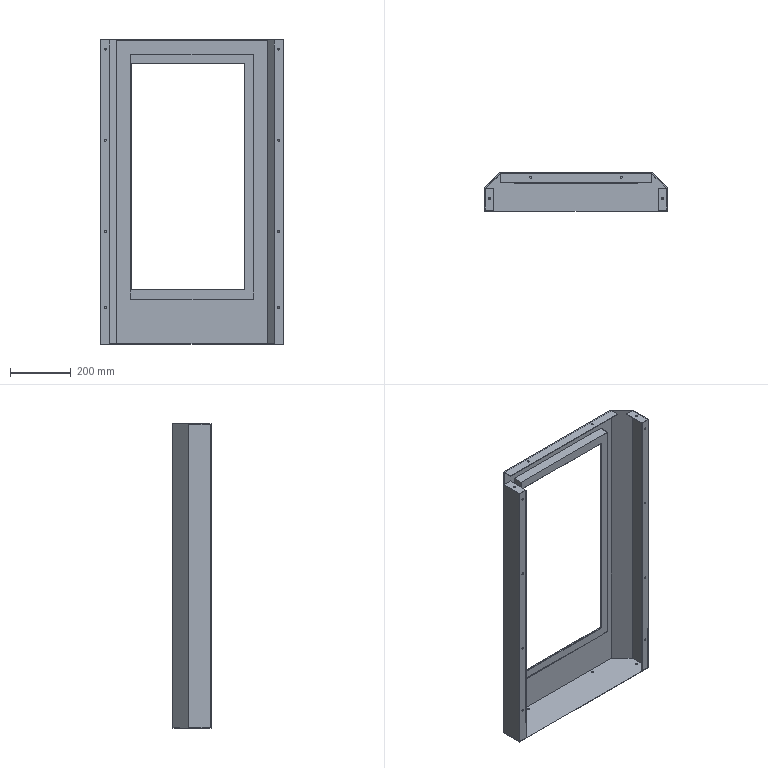Part | SolidWorks | features ICE 11, Extrusion 1, Shell 1 | 1 solid | 71 faces | box 600 x 125 x 1000 mm | volume 1467494 mm3 | plane 39 | cylinder 32 | commonest cylinder face diameters 6 x32